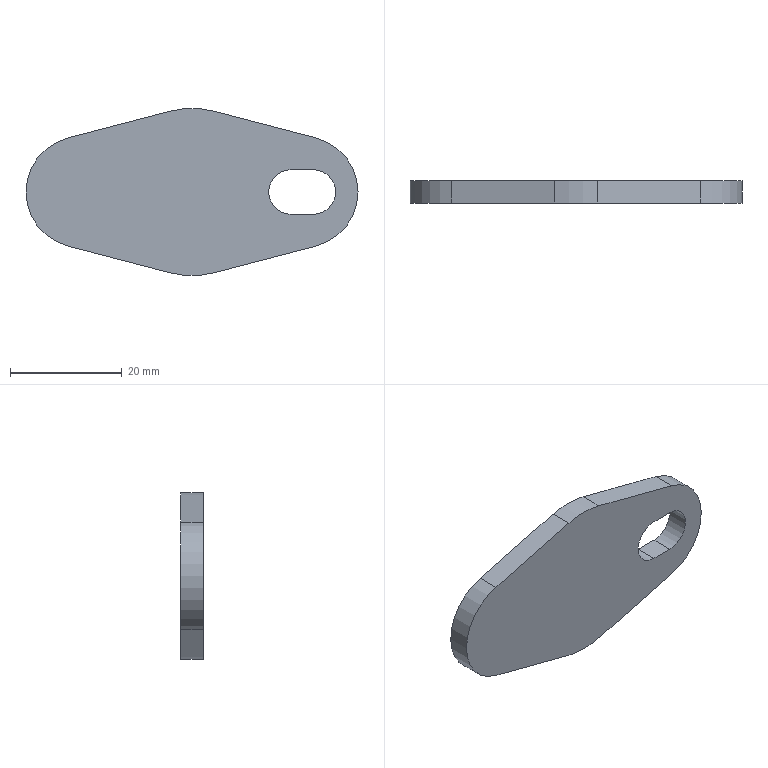Part | SolidWorks | features BaseBody 1 | 1 solid | 15 faces | box 59.526 x 4 x 30 mm | volume 5007 mm3 | plane 8 | cylinder 7 | commonest cylinder face diameters 20 x3 8 x2 30 x2
STEP:
#1=CARTESIAN_POINT('',(21.763,4.,4.));
#2=VERTEX_POINT('',#1);
#3=CARTESIAN_POINT('',(21.763,4.,-4.));
#4=VERTEX_POINT('',#3);
#5=CARTESIAN_POINT('',(21.763,4.,0.));
#6=DIRECTION('',(0.,1.,0.));
#7=DIRECTION('',(0.,0.,1.));
#8=AXIS2_PLACEMENT_3D('',#5,#6,#7);
#9=CIRCLE('',#8,4.);
#10=EDGE_CURVE('',#2,#4,#9,.T.);
#11=ORIENTED_EDGE('',*,*,#10,.F.);
#12=CARTESIAN_POINT('',(17.763,4.,4.));
#13=VERTEX_POINT('',#12);
#14=CARTESIAN_POINT('',(17.763,4.,4.));
#15=DIRECTION('',(1.,0.,0.));
#16=VECTOR('',#15,1000.);
#17=LINE('',#14,#16);
#18=EDGE_CURVE('',#13,#2,#17,.T.);
#19=ORIENTED_EDGE('',*,*,#18,.F.);
#20=CARTESIAN_POINT('',(17.763,4.,-4.));
#21=VERTEX_POINT('',#20);
#22=CARTESIAN_POINT('',(17.763,4.,0.));
#23=DIRECTION('',(0.,1.,0.));
#24=DIRECTION('',(0.,0.,-1.));
#25=AXIS2_PLACEMENT_3D('',#22,#23,#24);
#26=CIRCLE('',#25,4.);
#27=EDGE_CURVE('',#21,#13,#26,.T.);
#28=ORIENTED_EDGE('',*,*,#27,.F.);
#29=CARTESIAN_POINT('',(21.763,4.,-4.));
#30=DIRECTION('',(-1.,0.,0.));
#31=VECTOR('',#30,1000.);
#32=LINE('',#29,#31);
#33=EDGE_CURVE('',#4,#21,#32,.T.);
#34=ORIENTED_EDGE('',*,*,#33,.F.);
#35=EDGE_LOOP('',(#11,#19,#28,#34));
#36=FACE_BOUND('',#35,.T.);
#37=CARTESIAN_POINT('',(22.293,4.,-9.675));
#38=VERTEX_POINT('',#37);
#39=CARTESIAN_POINT('',(29.763,4.,0.));
#40=VERTEX_POINT('',#39);
#41=CARTESIAN_POINT('',(19.763,4.,0.));
#42=DIRECTION('',(0.,-1.,0.));
#43=DIRECTION('',(1.,0.,0.));
#44=AXIS2_PLACEMENT_3D('',#41,#42,#43);
#45=CIRCLE('',#44,10.);
#46=EDGE_CURVE('',#38,#40,#45,.T.);
#47=ORIENTED_EDGE('',*,*,#46,.F.);
#48=CARTESIAN_POINT('',(3.795,4.,-14.512));
#49=VERTEX_POINT('',#48);
#50=CARTESIAN_POINT('',(3.795,4.,-14.512));
#51=DIRECTION('',(0.9675,0.,0.253));
#52=VECTOR('',#51,1000.);
#53=LINE('',#50,#52);
#54=EDGE_CURVE('',#49,#38,#53,.T.);
#55=ORIENTED_EDGE('',*,*,#54,.F.);
#56=CARTESIAN_POINT('',(-3.795,4.,-14.512));
#57=VERTEX_POINT('',#56);
#58=CARTESIAN_POINT('',(0.,4.,0.));
#59=DIRECTION('',(0.,-1.,0.));
#60=DIRECTION('',(-0.253,0.,-0.9675));
#61=AXIS2_PLACEMENT_3D('',#58,#59,#60);
#62=CIRCLE('',#61,15.);
#63=EDGE_CURVE('',#57,#49,#62,.T.);
#64=ORIENTED_EDGE('',*,*,#63,.F.);
#65=CARTESIAN_POINT('',(-22.293,4.,-9.675));
#66=VERTEX_POINT('',#65);
#67=CARTESIAN_POINT('',(-22.293,4.,-9.675));
#68=DIRECTION('',(0.9675,0.,-0.253));
#69=VECTOR('',#68,1000.);
#70=LINE('',#67,#69);
#71=EDGE_CURVE('',#66,#57,#70,.T.);
#72=ORIENTED_EDGE('',*,*,#71,.F.);
#73=CARTESIAN_POINT('',(-22.293,4.,9.675));
#74=VERTEX_POINT('',#73);
#75=CARTESIAN_POINT('',(-19.763,4.,0.));
#76=DIRECTION('',(0.,-1.,0.));
#77=DIRECTION('',(-1.,0.,0.));
#78=AXIS2_PLACEMENT_3D('',#75,#76,#77);
#79=CIRCLE('',#78,10.);
#80=EDGE_CURVE('',#74,#66,#79,.T.);
#81=ORIENTED_EDGE('',*,*,#80,.F.);
#82=CARTESIAN_POINT('',(-3.795,4.,14.512));
#83=VERTEX_POINT('',#82);
#84=CARTESIAN_POINT('',(-3.795,4.,14.512));
#85=DIRECTION('',(-0.9675,0.,-0.253));
#86=VECTOR('',#85,1000.);
#87=LINE('',#84,#86);
#88=EDGE_CURVE('',#83,#74,#87,.T.);
#89=ORIENTED_EDGE('',*,*,#88,.F.);
#90=CARTESIAN_POINT('',(3.795,4.,14.512));
#91=VERTEX_POINT('',#90);
#92=CARTESIAN_POINT('',(0.,4.,0.));
#93=DIRECTION('',(0.,-1.,0.));
#94=DIRECTION('',(0.253,0.,0.9675));
#95=AXIS2_PLACEMENT_3D('',#92,#93,#94);
#96=CIRCLE('',#95,15.);
#97=EDGE_CURVE('',#91,#83,#96,.T.);
#98=ORIENTED_EDGE('',*,*,#97,.F.);
#99=CARTESIAN_POINT('',(22.293,4.,9.675));
#100=VERTEX_POINT('',#99);
#101=CARTESIAN_POINT('',(22.293,4.,9.675));
#102=DIRECTION('',(-0.9675,0.,0.253));
#103=VECTOR('',#102,1000.);
#104=LINE('',#101,#103);
#105=EDGE_CURVE('',#100,#91,#104,.T.);
#106=ORIENTED_EDGE('',*,*,#105,.F.);
#107=CARTESIAN_POINT('',(19.763,4.,0.));
#108=DIRECTION('',(0.,-1.,0.));
#109=DIRECTION('',(1.,0.,0.));
#110=AXIS2_PLACEMENT_3D('',#107,#108,#109);
#111=CIRCLE('',#110,10.);
#112=EDGE_CURVE('',#40,#100,#111,.T.);
#113=ORIENTED_EDGE('',*,*,#112,.F.);
#114=EDGE_LOOP('',(#47,#55,#64,#72,#81,#89,#98,#106,#113));
#115=FACE_OUTER_BOUND('',#114,.T.);
#116=CARTESIAN_POINT('',(0.,4.,0.));
#117=DIRECTION('',(0.,1.,0.));
#118=DIRECTION('',(1.,0.,0.));
#119=AXIS2_PLACEMENT_3D('',#116,#117,#118);
#120=PLANE('',#119);
#121=ADVANCED_FACE('',(#36,#115),#120,.T.);
#122=CARTESIAN_POINT('',(3.795,0.,14.512));
#123=VERTEX_POINT('',#122);
#124=CARTESIAN_POINT('',(3.795,4.,14.512));
#125=DIRECTION('',(0.,-1.,0.));
#126=VECTOR('',#125,1000.);
#127=LINE('',#124,#126);
#128=EDGE_CURVE('',#91,#123,#127,.T.);
#129=ORIENTED_EDGE('',*,*,#128,.T.);
#130=CARTESIAN_POINT('',(22.293,0.,9.675));
#131=VERTEX_POINT('',#130);
#132=CARTESIAN_POINT('',(3.795,0.,14.512));
#133=DIRECTION('',(0.9675,0.,-0.253));
#134=VECTOR('',#133,1000.);
#135=LINE('',#132,#134);
#136=EDGE_CURVE('',#123,#131,#135,.T.);
#137=ORIENTED_EDGE('',*,*,#136,.T.);
#138=CARTESIAN_POINT('',(22.293,0.,9.675));
#139=DIRECTION('',(0.,1.,0.));
#140=VECTOR('',#139,1000.);
#141=LINE('',#138,#140);
#142=EDGE_CURVE('',#131,#100,#141,.T.);
#143=ORIENTED_EDGE('',*,*,#142,.T.);
#144=ORIENTED_EDGE('',*,*,#105,.T.);
#145=EDGE_LOOP('',(#129,#137,#143,#144));
#146=FACE_OUTER_BOUND('',#145,.T.);
#147=CARTESIAN_POINT('',(22.293,4.,9.675));
#148=DIRECTION('',(-0.253,0.,-0.9675));
#149=DIRECTION('',(-0.9675,0.,0.253));
#150=AXIS2_PLACEMENT_3D('',#147,#148,#149);
#151=PLANE('',#150);
#152=ADVANCED_FACE('',(#146),#151,.F.);
#153=CARTESIAN_POINT('',(29.763,0.,0.));
#154=VERTEX_POINT('',#153);
#155=CARTESIAN_POINT('',(29.763,4.,0.));
#156=DIRECTION('',(0.,1.,0.));
#157=VECTOR('',#156,1000.);
#158=LINE('',#155,#157);
#159=EDGE_CURVE('',#154,#40,#158,.T.);
#160=ORIENTED_EDGE('',*,*,#159,.F.);
#161=CARTESIAN_POINT('',(22.293,0.,-9.675));
#162=VERTEX_POINT('',#161);
#163=CARTESIAN_POINT('',(19.763,0.,0.));
#164=DIRECTION('',(0.,1.,0.));
#165=DIRECTION('',(0.253,0.,0.9675));
#166=AXIS2_PLACEMENT_3D('',#163,#164,#165);
#167=CIRCLE('',#166,10.);
#168=EDGE_CURVE('',#154,#162,#167,.T.);
#169=ORIENTED_EDGE('',*,*,#168,.T.);
#170=CARTESIAN_POINT('',(22.293,4.,-9.675));
#171=DIRECTION('',(0.,-1.,0.));
#172=VECTOR('',#171,1000.);
#173=LINE('',#170,#172);
#174=EDGE_CURVE('',#38,#162,#173,.T.);
#175=ORIENTED_EDGE('',*,*,#174,.F.);
#176=ORIENTED_EDGE('',*,*,#46,.T.);
#177=EDGE_LOOP('',(#160,#169,#175,#176));
#178=FACE_OUTER_BOUND('',#177,.T.);
#179=CARTESIAN_POINT('',(19.763,4.,0.));
#180=DIRECTION('',(0.,1.,0.));
#181=DIRECTION('',(1.,0.,0.));
#182=AXIS2_PLACEMENT_3D('',#179,#180,#181);
#183=CYLINDRICAL_SURFACE('',#182,10.);
#184=ADVANCED_FACE('',(#178),#183,.T.);
#185=ORIENTED_EDGE('',*,*,#174,.T.);
#186=CARTESIAN_POINT('',(3.795,0.,-14.512));
#187=VERTEX_POINT('',#186);
#188=CARTESIAN_POINT('',(22.293,0.,-9.675));
#189=DIRECTION('',(-0.9675,0.,-0.253));
#190=VECTOR('',#189,1000.);
#191=LINE('',#188,#190);
#192=EDGE_CURVE('',#162,#187,#191,.T.);
#193=ORIENTED_EDGE('',*,*,#192,.T.);
#194=CARTESIAN_POINT('',(3.795,0.,-14.512));
#195=DIRECTION('',(0.,1.,0.));
#196=VECTOR('',#195,1000.);
#197=LINE('',#194,#196);
#198=EDGE_CURVE('',#187,#49,#197,.T.);
#199=ORIENTED_EDGE('',*,*,#198,.T.);
#200=ORIENTED_EDGE('',*,*,#54,.T.);
#201=EDGE_LOOP('',(#185,#193,#199,#200));
#202=FACE_OUTER_BOUND('',#201,.T.);
#203=CARTESIAN_POINT('',(3.795,4.,-14.512));
#204=DIRECTION('',(-0.253,0.,0.9675));
#205=DIRECTION('',(0.,1.,0.));
#206=AXIS2_PLACEMENT_3D('',#203,#204,#205);
#207=PLANE('',#206);
#208=ADVANCED_FACE('',(#202),#207,.F.);
#209=ORIENTED_EDGE('',*,*,#198,.F.);
#210=CARTESIAN_POINT('',(-3.795,0.,-14.512));
#211=VERTEX_POINT('',#210);
#212=CARTESIAN_POINT('',(0.,0.,0.));
#213=DIRECTION('',(0.,1.,0.));
#214=DIRECTION('',(0.253,0.,-0.9675));
#215=AXIS2_PLACEMENT_3D('',#212,#213,#214);
#216=CIRCLE('',#215,15.);
#217=EDGE_CURVE('',#187,#211,#216,.T.);
#218=ORIENTED_EDGE('',*,*,#217,.T.);
#219=CARTESIAN_POINT('',(-3.795,4.,-14.512));
#220=DIRECTION('',(0.,-1.,0.));
#221=VECTOR('',#220,1000.);
#222=LINE('',#219,#221);
#223=EDGE_CURVE('',#57,#211,#222,.T.);
#224=ORIENTED_EDGE('',*,*,#223,.F.);
#225=ORIENTED_EDGE('',*,*,#63,.T.);
#226=EDGE_LOOP('',(#209,#218,#224,#225));
#227=FACE_OUTER_BOUND('',#226,.T.);
#228=CARTESIAN_POINT('',(0.,4.,0.));
#229=DIRECTION('',(0.,1.,0.));
#230=DIRECTION('',(1.,0.,0.));
#231=AXIS2_PLACEMENT_3D('',#228,#229,#230);
#232=CYLINDRICAL_SURFACE('',#231,15.);
#233=ADVANCED_FACE('',(#227),#232,.T.);
#234=ORIENTED_EDGE('',*,*,#223,.T.);
#235=CARTESIAN_POINT('',(-22.293,0.,-9.675));
#236=VERTEX_POINT('',#235);
#237=CARTESIAN_POINT('',(-3.795,0.,-14.512));
#238=DIRECTION('',(-0.9675,0.,0.253));
#239=VECTOR('',#238,1000.);
#240=LINE('',#237,#239);
#241=EDGE_CURVE('',#211,#236,#240,.T.);
#242=ORIENTED_EDGE('',*,*,#241,.T.);
#243=CARTESIAN_POINT('',(-22.293,0.,-9.675));
#244=DIRECTION('',(0.,1.,0.));
#245=VECTOR('',#244,1000.);
#246=LINE('',#243,#245);
#247=EDGE_CURVE('',#236,#66,#246,.T.);
#248=ORIENTED_EDGE('',*,*,#247,.T.);
#249=ORIENTED_EDGE('',*,*,#71,.T.);
#250=EDGE_LOOP('',(#234,#242,#248,#249));
#251=FACE_OUTER_BOUND('',#250,.T.);
#252=CARTESIAN_POINT('',(-22.293,4.,-9.675));
#253=DIRECTION('',(0.253,0.,0.9675));
#254=DIRECTION('',(0.,-1.,0.));
#255=AXIS2_PLACEMENT_3D('',#252,#253,#254);
#256=PLANE('',#255);
#257=ADVANCED_FACE('',(#251),#256,.F.);
#258=ORIENTED_EDGE('',*,*,#247,.F.);
#259=CARTESIAN_POINT('',(-22.293,0.,9.675));
#260=VERTEX_POINT('',#259);
#261=CARTESIAN_POINT('',(-19.763,0.,0.));
#262=DIRECTION('',(0.,1.,0.));
#263=DIRECTION('',(-0.253,0.,-0.9675));
#264=AXIS2_PLACEMENT_3D('',#261,#262,#263);
#265=CIRCLE('',#264,10.);
#266=EDGE_CURVE('',#236,#260,#265,.T.);
#267=ORIENTED_EDGE('',*,*,#266,.T.);
#268=CARTESIAN_POINT('',(-22.293,4.,9.675));
#269=DIRECTION('',(0.,-1.,0.));
#270=VECTOR('',#269,1000.);
#271=LINE('',#268,#270);
#272=EDGE_CURVE('',#74,#260,#271,.T.);
#273=ORIENTED_EDGE('',*,*,#272,.F.);
#274=ORIENTED_EDGE('',*,*,#80,.T.);
#275=EDGE_LOOP('',(#258,#267,#273,#274));
#276=FACE_OUTER_BOUND('',#275,.T.);
#277=CARTESIAN_POINT('',(-19.763,4.,0.));
#278=DIRECTION('',(0.,1.,0.));
#279=DIRECTION('',(1.,0.,0.));
#280=AXIS2_PLACEMENT_3D('',#277,#278,#279);
#281=CYLINDRICAL_SURFACE('',#280,10.);
#282=ADVANCED_FACE('',(#276),#281,.T.);
#283=ORIENTED_EDGE('',*,*,#272,.T.);
#284=CARTESIAN_POINT('',(-3.795,0.,14.512));
#285=VERTEX_POINT('',#284);
#286=CARTESIAN_POINT('',(-22.293,0.,9.675));
#287=DIRECTION('',(0.9675,0.,0.253));
#288=VECTOR('',#287,1000.);
#289=LINE('',#286,#288);
#290=EDGE_CURVE('',#260,#285,#289,.T.);
#291=ORIENTED_EDGE('',*,*,#290,.T.);
#292=CARTESIAN_POINT('',(-3.795,0.,14.512));
#293=DIRECTION('',(0.,1.,0.));
#294=VECTOR('',#293,1000.);
#295=LINE('',#292,#294);
#296=EDGE_CURVE('',#285,#83,#295,.T.);
#297=ORIENTED_EDGE('',*,*,#296,.T.);
#298=ORIENTED_EDGE('',*,*,#88,.T.);
#299=EDGE_LOOP('',(#283,#291,#297,#298));
#300=FACE_OUTER_BOUND('',#299,.T.);
#301=CARTESIAN_POINT('',(-3.795,4.,14.512));
#302=DIRECTION('',(0.253,0.,-0.9675));
#303=DIRECTION('',(0.,-1.,0.));
#304=AXIS2_PLACEMENT_3D('',#301,#302,#303);
#305=PLANE('',#304);
#306=ADVANCED_FACE('',(#300),#305,.F.);
#307=ORIENTED_EDGE('',*,*,#296,.F.);
#308=CARTESIAN_POINT('',(0.,0.,0.));
#309=DIRECTION('',(0.,1.,0.));
#310=DIRECTION('',(-0.253,0.,0.9675));
#311=AXIS2_PLACEMENT_3D('',#308,#309,#310);
#312=CIRCLE('',#311,15.);
#313=EDGE_CURVE('',#285,#123,#312,.T.);
#314=ORIENTED_EDGE('',*,*,#313,.T.);
#315=ORIENTED_EDGE('',*,*,#128,.F.);
#316=ORIENTED_EDGE('',*,*,#97,.T.);
#317=EDGE_LOOP('',(#307,#314,#315,#316));
#318=FACE_OUTER_BOUND('',#317,.T.);
#319=CARTESIAN_POINT('',(0.,4.,0.));
#320=DIRECTION('',(0.,1.,0.));
#321=DIRECTION('',(1.,0.,0.));
#322=AXIS2_PLACEMENT_3D('',#319,#320,#321);
#323=CYLINDRICAL_SURFACE('',#322,15.);
#324=ADVANCED_FACE('',(#318),#323,.T.);
#325=CARTESIAN_POINT('',(17.763,0.,4.));
#326=VERTEX_POINT('',#325);
#327=CARTESIAN_POINT('',(17.763,0.,-4.));
#328=VERTEX_POINT('',#327);
#329=CARTESIAN_POINT('',(17.763,0.,0.));
#330=DIRECTION('',(0.,-1.,0.));
#331=DIRECTION('',(0.,0.,1.));
#332=AXIS2_PLACEMENT_3D('',#329,#330,#331);
#333=CIRCLE('',#332,4.);
#334=EDGE_CURVE('',#326,#328,#333,.T.);
#335=ORIENTED_EDGE('',*,*,#334,.F.);
#336=CARTESIAN_POINT('',(21.763,0.,4.));
#337=VERTEX_POINT('',#336);
#338=CARTESIAN_POINT('',(17.763,0.,4.));
#339=DIRECTION('',(1.,0.,0.));
#340=VECTOR('',#339,1000.);
#341=LINE('',#338,#340);
#342=EDGE_CURVE('',#326,#337,#341,.T.);
#343=ORIENTED_EDGE('',*,*,#342,.T.);
#344=CARTESIAN_POINT('',(21.763,0.,-4.));
#345=VERTEX_POINT('',#344);
#346=CARTESIAN_POINT('',(21.763,0.,0.));
#347=DIRECTION('',(0.,-1.,0.));
#348=DIRECTION('',(0.,0.,-1.));
#349=AXIS2_PLACEMENT_3D('',#346,#347,#348);
#350=CIRCLE('',#349,4.);
#351=EDGE_CURVE('',#345,#337,#350,.T.);
#352=ORIENTED_EDGE('',*,*,#351,.F.);
#353=CARTESIAN_POINT('',(21.763,0.,-4.));
#354=DIRECTION('',(-1.,0.,0.));
#355=VECTOR('',#354,1000.);
#356=LINE('',#353,#355);
#357=EDGE_CURVE('',#345,#328,#356,.T.);
#358=ORIENTED_EDGE('',*,*,#357,.T.);
#359=EDGE_LOOP('',(#335,#343,#352,#358));
#360=FACE_BOUND('',#359,.T.);
#361=ORIENTED_EDGE('',*,*,#313,.F.);
#362=ORIENTED_EDGE('',*,*,#290,.F.);
#363=ORIENTED_EDGE('',*,*,#266,.F.);
#364=ORIENTED_EDGE('',*,*,#241,.F.);
#365=ORIENTED_EDGE('',*,*,#217,.F.);
#366=ORIENTED_EDGE('',*,*,#192,.F.);
#367=ORIENTED_EDGE('',*,*,#168,.F.);
#368=CARTESIAN_POINT('',(19.763,0.,0.));
#369=DIRECTION('',(0.,1.,0.));
#370=DIRECTION('',(0.253,0.,0.9675));
#371=AXIS2_PLACEMENT_3D('',#368,#369,#370);
#372=CIRCLE('',#371,10.);
#373=EDGE_CURVE('',#131,#154,#372,.T.);
#374=ORIENTED_EDGE('',*,*,#373,.F.);
#375=ORIENTED_EDGE('',*,*,#136,.F.);
#376=EDGE_LOOP('',(#361,#362,#363,#364,#365,#366,#367,#374,#375));
#377=FACE_OUTER_BOUND('',#376,.T.);
#378=CARTESIAN_POINT('',(0.,0.,0.));
#379=DIRECTION('',(0.,1.,0.));
#380=DIRECTION('',(1.,0.,0.));
#381=AXIS2_PLACEMENT_3D('',#378,#379,#380);
#382=PLANE('',#381);
#383=ADVANCED_FACE('',(#360,#377),#382,.F.);
#384=CARTESIAN_POINT('',(17.763,4.,-4.));
#385=DIRECTION('',(0.,-1.,0.));
#386=VECTOR('',#385,1000.);
#387=LINE('',#384,#386);
#388=EDGE_CURVE('',#21,#328,#387,.T.);
#389=ORIENTED_EDGE('',*,*,#388,.T.);
#390=ORIENTED_EDGE('',*,*,#357,.F.);
#391=CARTESIAN_POINT('',(21.763,0.,-4.));
#392=DIRECTION('',(0.,1.,0.));
#393=VECTOR('',#392,1000.);
#394=LINE('',#391,#393);
#395=EDGE_CURVE('',#345,#4,#394,.T.);
#396=ORIENTED_EDGE('',*,*,#395,.T.);
#397=ORIENTED_EDGE('',*,*,#33,.T.);
#398=EDGE_LOOP('',(#389,#390,#396,#397));
#399=FACE_OUTER_BOUND('',#398,.T.);
#400=CARTESIAN_POINT('',(19.763,2.,-4.));
#401=DIRECTION('',(0.,0.,1.));
#402=DIRECTION('',(1.,0.,0.));
#403=AXIS2_PLACEMENT_3D('',#400,#401,#402);
#404=PLANE('',#403);
#405=ADVANCED_FACE('',(#399),#404,.T.);
#406=ORIENTED_EDGE('',*,*,#395,.F.);
#407=ORIENTED_EDGE('',*,*,#351,.T.);
#408=CARTESIAN_POINT('',(21.763,4.,4.));
#409=DIRECTION('',(0.,-1.,0.));
#410=VECTOR('',#409,1000.);
#411=LINE('',#408,#410);
#412=EDGE_CURVE('',#2,#337,#411,.T.);
#413=ORIENTED_EDGE('',*,*,#412,.F.);
#414=ORIENTED_EDGE('',*,*,#10,.T.);
#415=EDGE_LOOP('',(#406,#407,#413,#414));
#416=FACE_OUTER_BOUND('',#415,.T.);
#417=CARTESIAN_POINT('',(21.763,2.,0.));
#418=DIRECTION('',(0.,-1.,0.));
#419=DIRECTION('',(0.,0.,-1.));
#420=AXIS2_PLACEMENT_3D('',#417,#418,#419);
#421=CYLINDRICAL_SURFACE('',#420,4.);
#422=ADVANCED_FACE('',(#416),#421,.F.);
#423=ORIENTED_EDGE('',*,*,#412,.T.);
#424=ORIENTED_EDGE('',*,*,#342,.F.);
#425=CARTESIAN_POINT('',(17.763,0.,4.));
#426=DIRECTION('',(0.,1.,0.));
#427=VECTOR('',#426,1000.);
#428=LINE('',#425,#427);
#429=EDGE_CURVE('',#326,#13,#428,.T.);
#430=ORIENTED_EDGE('',*,*,#429,.T.);
#431=ORIENTED_EDGE('',*,*,#18,.T.);
#432=EDGE_LOOP('',(#423,#424,#430,#431));
#433=FACE_OUTER_BOUND('',#432,.T.);
#434=CARTESIAN_POINT('',(19.763,2.,4.));
#435=DIRECTION('',(0.,0.,-1.));
#436=DIRECTION('',(0.,-1.,0.));
#437=AXIS2_PLACEMENT_3D('',#434,#435,#436);
#438=PLANE('',#437);
#439=ADVANCED_FACE('',(#433),#438,.T.);
#440=ORIENTED_EDGE('',*,*,#429,.F.);
#441=ORIENTED_EDGE('',*,*,#334,.T.);
#442=ORIENTED_EDGE('',*,*,#388,.F.);
#443=ORIENTED_EDGE('',*,*,#27,.T.);
#444=EDGE_LOOP('',(#440,#441,#442,#443));
#445=FACE_OUTER_BOUND('',#444,.T.);
#446=CARTESIAN_POINT('',(17.763,2.,0.));
#447=DIRECTION('',(0.,-1.,0.));
#448=DIRECTION('',(0.,0.,1.));
#449=AXIS2_PLACEMENT_3D('',#446,#447,#448);
#450=CYLINDRICAL_SURFACE('',#449,4.);
#451=ADVANCED_FACE('',(#445),#450,.F.);
#452=ORIENTED_EDGE('',*,*,#373,.T.);
#453=ORIENTED_EDGE('',*,*,#159,.T.);
#454=ORIENTED_EDGE('',*,*,#112,.T.);
#455=ORIENTED_EDGE('',*,*,#142,.F.);
#456=EDGE_LOOP('',(#452,#453,#454,#455));
#457=FACE_OUTER_BOUND('',#456,.T.);
#458=CARTESIAN_POINT('',(19.763,4.,0.));
#459=DIRECTION('',(0.,1.,0.));
#460=DIRECTION('',(1.,0.,0.));
#461=AXIS2_PLACEMENT_3D('',#458,#459,#460);
#462=CYLINDRICAL_SURFACE('',#461,10.);
#463=ADVANCED_FACE('',(#457),#462,.T.);
#464=CLOSED_SHELL('',(#121,#152,#184,#208,#233,#257,#282,#306,#324,#383,#405,#422,#439,#451,#463));
#465=MANIFOLD_SOLID_BREP('',#464);
#466=CARTESIAN_POINT('',(0.,0.,0.));
#467=DIRECTION('',(0.,0.,1.));
#468=DIRECTION('',(1.,0.,0.));
#469=AXIS2_PLACEMENT_3D('',#466,#467,#468);
#470=(LENGTH_UNIT()NAMED_UNIT(*)SI_UNIT(.MILLI.,.METRE.));
#471=UNCERTAINTY_MEASURE_WITH_UNIT(LENGTH_MEASURE(0.00001),#470,'','');
#472=(NAMED_UNIT(*)PLANE_ANGLE_UNIT()SI_UNIT($,.RADIAN.));
#473=(NAMED_UNIT(*)SI_UNIT($,.STERADIAN.)SOLID_ANGLE_UNIT());
#474=(GEOMETRIC_REPRESENTATION_CONTEXT(3)GLOBAL_UNCERTAINTY_ASSIGNED_CONTEXT((#471))GLOBAL_UNIT_ASSIGNED_CONTEXT((#470,#472,#473))REPRESENTATION_CONTEXT('',''));
#475=ADVANCED_BREP_SHAPE_REPRESENTATION('',(#465,#469),#474);